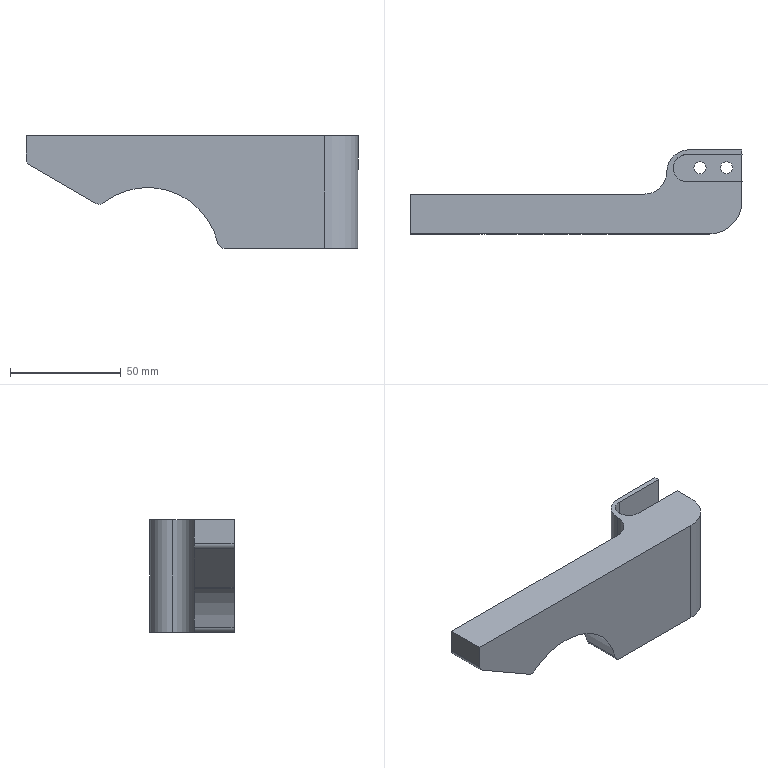NC program | NX | posted with a generic post | part box 150 x 38 x 51 mm
Lines 1 to 45 of 31037:
N10 G17 G21 G94 G90
(FLOOR_WALL , TOOL : D63)
N12 T01 M6
N14 G54
N16 G17 G0 G90 X114.5 Y-23.997 S6500 M3
N18 G43 Z30. H1
N20 Z3.
N22 G94 G1 Z0. F1500.
N24 X111.5
N26 X-111.5
N28 Y-13.786
N30 Y-1.2
N32 X111.5
N34 X114.5
N36 Z3.
N38 G0 Z30.
N40 M5
(DRILLING , TOOL : D6A45)
N42 T07 M6
N44 G54
N46 G17 G0 G90 X68. Y-10.9 S5000 M3
N48 G43 Z30. H7
N50 G94 G81 G98 Z-1. F250. R3.
N52 X56.
N54 G80
N56 G0 X56. Y-10.9 Z30.
N58 M5
(DRILLING_COPY , TOOL : 5.5ZT)
N60 T15 M6
N62 G54
N64 G17 G0 G90 X56. Y-10.9 S2000 M3
N66 G43 Z30. H15
N68 G94 G83 G98 Z-41.652 F200. Q2. R3.
N70 X68.
N72 G80
N74 G0 X68. Y-10.9 Z30.
N76 M5